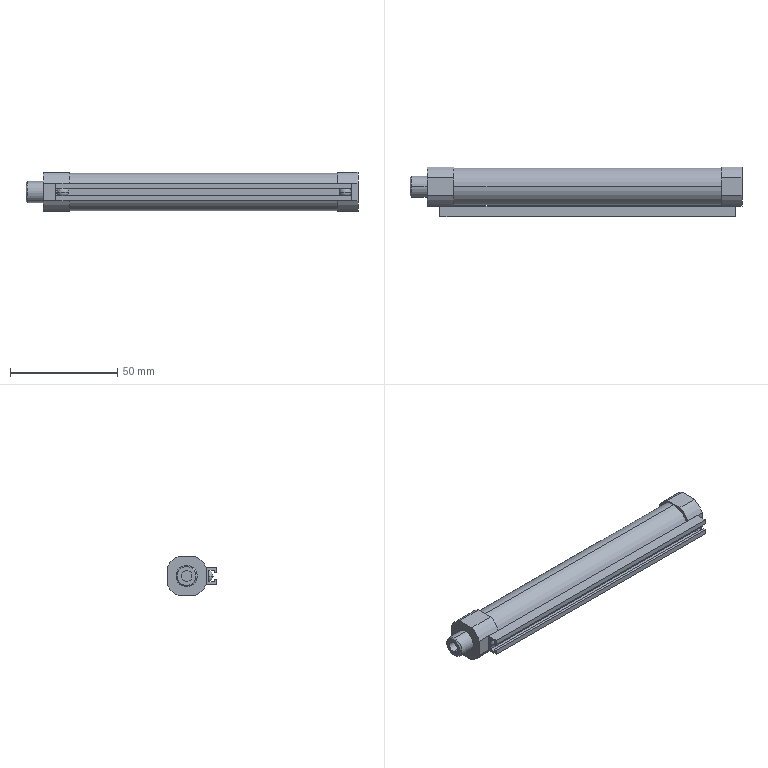Part | SolidWorks | features RefAxis 21, 3DProfileFeature 7, ICE 4, HoleWzd 2, Revolution 2, LPattern 1, RevCut 1 | 1 solid | 63 faces | box 155 x 23.3 x 18.3 mm | volume 18210 mm3 | plane 29 | cylinder 20 | cone 10 | sphere 4 | commonest cylinder face diameters 20 x8 4.134 x4 5 x2 10 x2 16 x2 17.4 x2